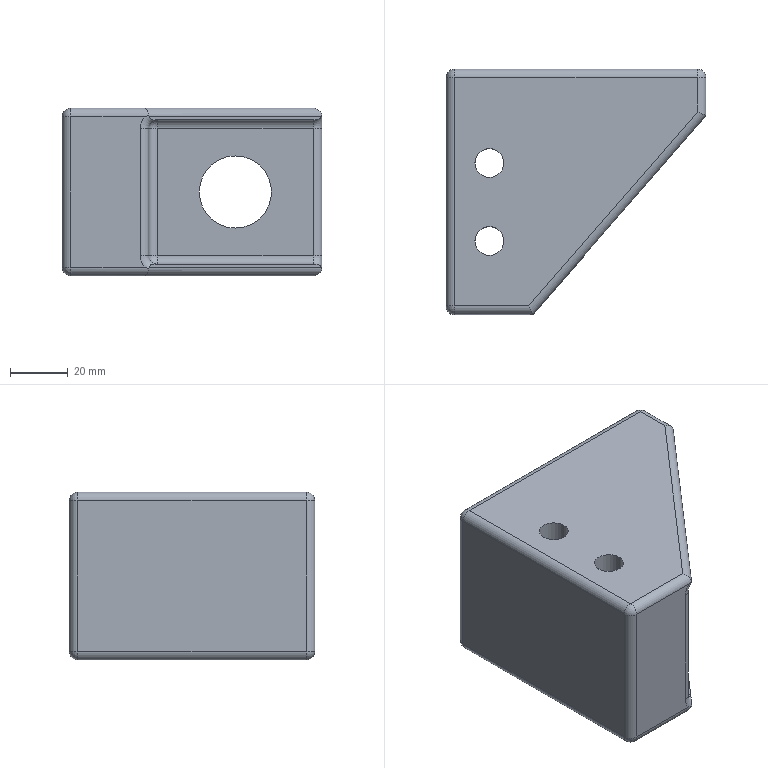Part | SolidWorks | features Fillet 3, ICE 3, Extrusion 1, MirrorPattern 1 | 1 solid | 54 faces | box 90 x 85 x 58 mm | volume 199222 mm3 | cylinder 28 | plane 13 | sphere 8 | torus 5 | commonest cylinder face diameters 6 x20 10 x4 12 x2 25 x2